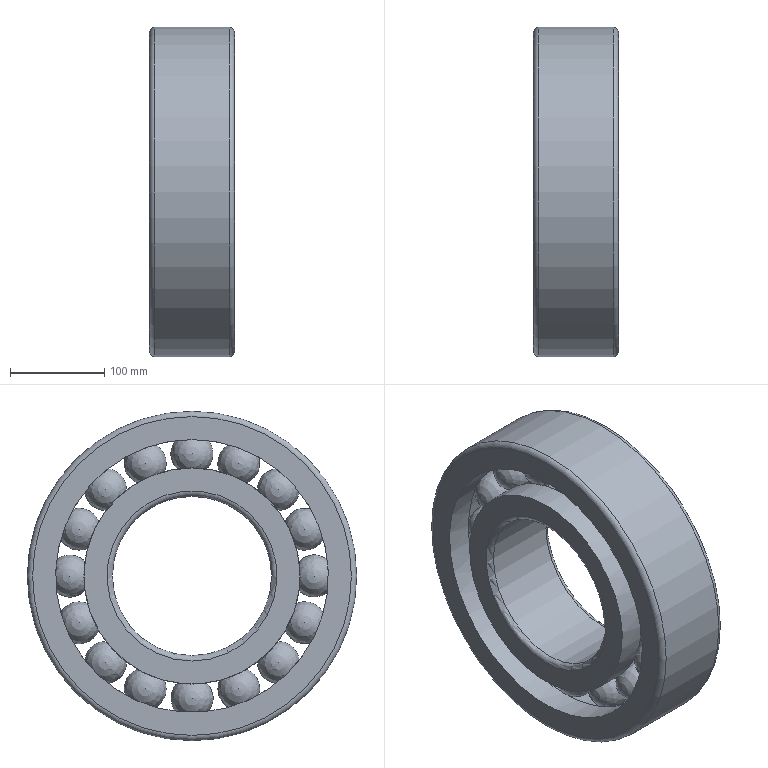Part | NX | features 25.SLDPRT 2, Delete Body 1, LINKED_BODY 1, SCALE 1 | 1 solid | 62 faces | box 90 x 348.75 x 348.75 mm | volume 4853865 mm3 | torus 36 | sphere 16 | cylinder 6 | plane 4 | commonest cylinder face diameters 228.75 x2 288.75 x2 168.75 x1 348.75 x1